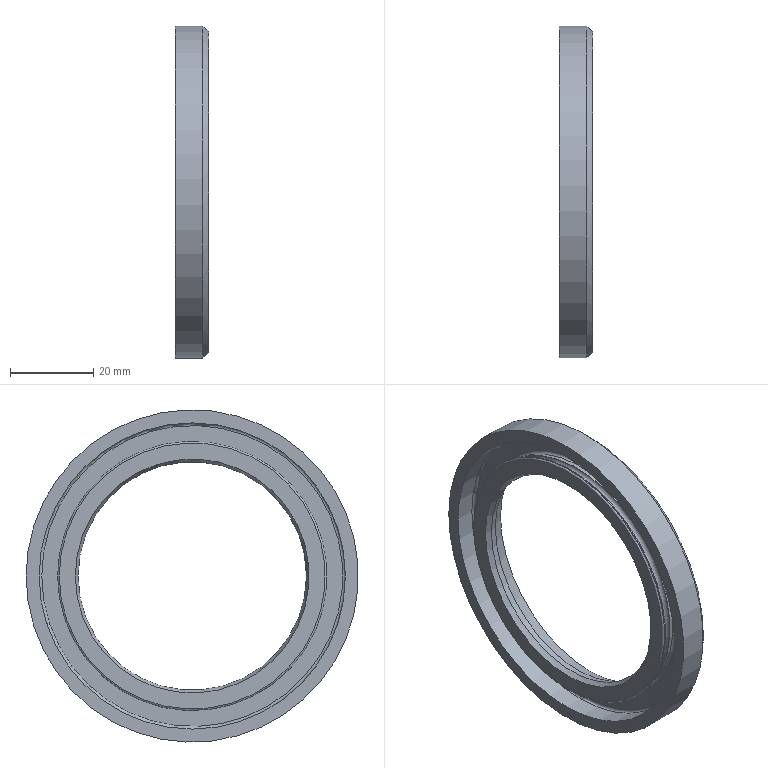Part | STEP file | Housing | 1 solid | 31 faces | box 8 x 80 x 80 mm | volume 10893 mm3 | plane 11 | cylinder 9 | torus 7 | cone 4 | commonest cylinder face diameters 67.5 x2 63.25 x1 64.85 x1 71.75 x1 73.75 x1 76.597 x1
STEP:
#1=CARTESIAN_POINT('',(8.,33.75,0.));
#2=VERTEX_POINT('',#1);
#3=CARTESIAN_POINT('',(8.,0.,0.));
#4=DIRECTION('',(1.,0.,0.));
#5=DIRECTION('',(0.,1.,0.));
#6=AXIS2_PLACEMENT_3D('',#3,#4,#5);
#7=CIRCLE('',#6,33.75);
#8=EDGE_CURVE('',#2,#2,#7,.T.);
#9=ORIENTED_EDGE('',*,*,#8,.T.);
#10=EDGE_LOOP('',(#9));
#11=FACE_BOUND('',#10,.T.);
#12=CARTESIAN_POINT('',(8.,30.393,0.));
#13=VERTEX_POINT('',#12);
#14=CARTESIAN_POINT('',(8.,0.,0.));
#15=DIRECTION('',(1.,0.,0.));
#16=DIRECTION('',(0.,1.,0.));
#17=AXIS2_PLACEMENT_3D('',#14,#15,#16);
#18=CIRCLE('',#17,30.393);
#19=EDGE_CURVE('',#13,#13,#18,.F.);
#20=ORIENTED_EDGE('',*,*,#19,.T.);
#21=EDGE_LOOP('',(#20));
#22=FACE_BOUND('',#21,.T.);
#23=CARTESIAN_POINT('',(8.,0.,0.));
#24=DIRECTION('',(1.,0.,0.));
#25=DIRECTION('',(0.,1.,0.));
#26=AXIS2_PLACEMENT_3D('',#23,#24,#25);
#27=PLANE('',#26);
#28=ADVANCED_FACE('',(#11,#22),#27,.T.);
#29=CARTESIAN_POINT('',(4.,28.15,0.));
#30=VERTEX_POINT('',#29);
#31=CARTESIAN_POINT('',(4.,0.,0.));
#32=DIRECTION('',(1.,0.,0.));
#33=DIRECTION('',(0.,1.,0.));
#34=AXIS2_PLACEMENT_3D('',#31,#32,#33);
#35=CIRCLE('',#34,28.15);
#36=EDGE_CURVE('',#30,#30,#35,.T.);
#37=ORIENTED_EDGE('',*,*,#36,.T.);
#38=EDGE_LOOP('',(#37));
#39=FACE_OUTER_BOUND('',#38,.T.);
#40=CARTESIAN_POINT('',(2.,27.5,0.));
#41=VERTEX_POINT('',#40);
#42=CARTESIAN_POINT('',(2.,0.,0.));
#43=DIRECTION('',(1.,0.,0.));
#44=DIRECTION('',(0.,1.,0.));
#45=AXIS2_PLACEMENT_3D('',#42,#43,#44);
#46=CIRCLE('',#45,27.5);
#47=EDGE_CURVE('',#41,#41,#46,.T.);
#48=ORIENTED_EDGE('',*,*,#47,.F.);
#49=EDGE_LOOP('',(#48));
#50=FACE_OUTER_BOUND('',#49,.T.);
#51=CARTESIAN_POINT('',(3.,0.,0.));
#52=DIRECTION('',(1.,0.,0.));
#53=DIRECTION('',(0.,1.,0.));
#54=AXIS2_PLACEMENT_3D('',#51,#52,#53);
#55=CONICAL_SURFACE('',#54,27.825,0.3142);
#56=ADVANCED_FACE('',(#39,#50),#55,.F.);
#57=CARTESIAN_POINT('',(4.,28.442,0.));
#58=VERTEX_POINT('',#57);
#59=CARTESIAN_POINT('',(4.,0.,0.));
#60=DIRECTION('',(1.,0.,0.));
#61=DIRECTION('',(0.,1.,0.));
#62=AXIS2_PLACEMENT_3D('',#59,#60,#61);
#63=CIRCLE('',#62,28.442);
#64=EDGE_CURVE('',#58,#58,#63,.T.);
#65=ORIENTED_EDGE('',*,*,#64,.T.);
#66=EDGE_LOOP('',(#65));
#67=FACE_BOUND('',#66,.T.);
#68=ORIENTED_EDGE('',*,*,#36,.F.);
#69=EDGE_LOOP('',(#68));
#70=FACE_BOUND('',#69,.T.);
#71=CARTESIAN_POINT('',(4.,0.,0.));
#72=DIRECTION('',(-1.,0.,0.));
#73=DIRECTION('',(0.,1.,0.));
#74=AXIS2_PLACEMENT_3D('',#71,#72,#73);
#75=PLANE('',#74);
#76=ADVANCED_FACE('',(#67,#70),#75,.F.);
#77=ORIENTED_EDGE('',*,*,#19,.F.);
#78=EDGE_LOOP('',(#77));
#79=FACE_OUTER_BOUND('',#78,.T.);
#80=ORIENTED_EDGE('',*,*,#64,.F.);
#81=EDGE_LOOP('',(#80));
#82=FACE_OUTER_BOUND('',#81,.T.);
#83=CARTESIAN_POINT('',(6.,0.,0.));
#84=DIRECTION('',(1.,0.,0.));
#85=DIRECTION('',(0.,1.,0.));
#86=AXIS2_PLACEMENT_3D('',#83,#84,#85);
#87=CONICAL_SURFACE('',#86,29.418,0.4538);
#88=ADVANCED_FACE('',(#79,#82),#87,.F.);
#89=ORIENTED_EDGE('',*,*,#8,.F.);
#90=EDGE_LOOP('',(#89));
#91=FACE_OUTER_BOUND('',#90,.T.);
#92=CARTESIAN_POINT('',(7.36,33.75,0.));
#93=VERTEX_POINT('',#92);
#94=CARTESIAN_POINT('',(7.36,0.,0.));
#95=DIRECTION('',(1.,0.,0.));
#96=DIRECTION('',(0.,1.,0.));
#97=AXIS2_PLACEMENT_3D('',#94,#95,#96);
#98=CIRCLE('',#97,33.75);
#99=EDGE_CURVE('',#93,#93,#98,.T.);
#100=ORIENTED_EDGE('',*,*,#99,.T.);
#101=EDGE_LOOP('',(#100));
#102=FACE_OUTER_BOUND('',#101,.T.);
#103=CARTESIAN_POINT('',(8.,0.,0.));
#104=DIRECTION('',(1.,0.,0.));
#105=DIRECTION('',(0.,1.,0.));
#106=AXIS2_PLACEMENT_3D('',#103,#104,#105);
#107=CYLINDRICAL_SURFACE('',#106,33.75);
#108=ADVANCED_FACE('',(#91,#102),#107,.T.);
#109=ORIENTED_EDGE('',*,*,#47,.T.);
#110=EDGE_LOOP('',(#109));
#111=FACE_OUTER_BOUND('',#110,.T.);
#112=CARTESIAN_POINT('',(0.64,28.163,0.));
#113=VERTEX_POINT('',#112);
#114=CARTESIAN_POINT('',(0.64,0.,0.));
#115=DIRECTION('',(1.,0.,0.));
#116=DIRECTION('',(0.,1.,0.));
#117=AXIS2_PLACEMENT_3D('',#114,#115,#116);
#118=CIRCLE('',#117,28.163);
#119=EDGE_CURVE('',#113,#113,#118,.T.);
#120=ORIENTED_EDGE('',*,*,#119,.F.);
#121=EDGE_LOOP('',(#120));
#122=FACE_OUTER_BOUND('',#121,.T.);
#123=CARTESIAN_POINT('',(1.32,0.,0.));
#124=DIRECTION('',(-1.,0.,0.));
#125=DIRECTION('',(0.,-1.,0.));
#126=AXIS2_PLACEMENT_3D('',#123,#124,#125);
#127=CONICAL_SURFACE('',#126,27.832,0.4538);
#128=ADVANCED_FACE('',(#111,#122),#127,.F.);
#129=CARTESIAN_POINT('',(7.36,35.875,0.));
#130=VERTEX_POINT('',#129);
#131=CARTESIAN_POINT('',(7.36,0.,0.));
#132=DIRECTION('',(1.,0.,0.));
#133=DIRECTION('',(0.,1.,0.));
#134=AXIS2_PLACEMENT_3D('',#131,#132,#133);
#135=CIRCLE('',#134,35.875);
#136=EDGE_CURVE('',#130,#130,#135,.T.);
#137=ORIENTED_EDGE('',*,*,#136,.T.);
#138=EDGE_LOOP('',(#137));
#139=FACE_BOUND('',#138,.T.);
#140=ORIENTED_EDGE('',*,*,#99,.F.);
#141=EDGE_LOOP('',(#140));
#142=FACE_BOUND('',#141,.T.);
#143=CARTESIAN_POINT('',(7.36,0.,0.));
#144=DIRECTION('',(-1.,0.,0.));
#145=DIRECTION('',(0.,1.,0.));
#146=AXIS2_PLACEMENT_3D('',#143,#144,#145);
#147=PLANE('',#146);
#148=ADVANCED_FACE('',(#139,#142),#147,.F.);
#149=CARTESIAN_POINT('',(0.64,32.025,0.));
#150=VERTEX_POINT('',#149);
#151=CARTESIAN_POINT('',(0.64,0.,0.));
#152=DIRECTION('',(1.,0.,0.));
#153=DIRECTION('',(0.,1.,0.));
#154=AXIS2_PLACEMENT_3D('',#151,#152,#153);
#155=CIRCLE('',#154,32.025);
#156=EDGE_CURVE('',#150,#150,#155,.T.);
#157=ORIENTED_EDGE('',*,*,#156,.F.);
#158=EDGE_LOOP('',(#157));
#159=FACE_BOUND('',#158,.T.);
#160=ORIENTED_EDGE('',*,*,#119,.T.);
#161=EDGE_LOOP('',(#160));
#162=FACE_BOUND('',#161,.T.);
#163=CARTESIAN_POINT('',(0.64,0.,0.));
#164=DIRECTION('',(1.,0.,0.));
#165=DIRECTION('',(0.,1.,0.));
#166=AXIS2_PLACEMENT_3D('',#163,#164,#165);
#167=PLANE('',#166);
#168=ADVANCED_FACE('',(#159,#162),#167,.F.);
#169=CARTESIAN_POINT('',(8.,35.875,0.));
#170=VERTEX_POINT('',#169);
#171=CARTESIAN_POINT('',(8.,0.,0.));
#172=DIRECTION('',(1.,0.,0.));
#173=DIRECTION('',(0.,1.,0.));
#174=AXIS2_PLACEMENT_3D('',#171,#172,#173);
#175=CIRCLE('',#174,35.875);
#176=EDGE_CURVE('',#170,#170,#175,.F.);
#177=ORIENTED_EDGE('',*,*,#176,.F.);
#178=EDGE_LOOP('',(#177));
#179=FACE_OUTER_BOUND('',#178,.T.);
#180=ORIENTED_EDGE('',*,*,#136,.F.);
#181=EDGE_LOOP('',(#180));
#182=FACE_OUTER_BOUND('',#181,.T.);
#183=CARTESIAN_POINT('',(7.36,0.,0.));
#184=DIRECTION('',(1.,0.,0.));
#185=DIRECTION('',(0.,1.,0.));
#186=AXIS2_PLACEMENT_3D('',#183,#184,#185);
#187=CYLINDRICAL_SURFACE('',#186,35.875);
#188=ADVANCED_FACE('',(#179,#182),#187,.F.);
#189=CARTESIAN_POINT('',(1.04,32.425,0.));
#190=VERTEX_POINT('',#189);
#191=CARTESIAN_POINT('',(1.04,0.,0.));
#192=DIRECTION('',(1.,0.,0.));
#193=DIRECTION('',(0.,1.,0.));
#194=AXIS2_PLACEMENT_3D('',#191,#192,#193);
#195=CIRCLE('',#194,32.425);
#196=EDGE_CURVE('',#190,#190,#195,.T.);
#197=ORIENTED_EDGE('',*,*,#196,.F.);
#198=EDGE_LOOP('',(#197));
#199=FACE_OUTER_BOUND('',#198,.T.);
#200=ORIENTED_EDGE('',*,*,#156,.T.);
#201=EDGE_LOOP('',(#200));
#202=FACE_OUTER_BOUND('',#201,.T.);
#203=CARTESIAN_POINT('',(1.04,0.,0.));
#204=DIRECTION('',(1.,0.,0.));
#205=DIRECTION('',(0.,1.,0.));
#206=AXIS2_PLACEMENT_3D('',#203,#204,#205);
#207=TOROIDAL_SURFACE('',#206,32.025,0.4);
#208=ADVANCED_FACE('',(#199,#202),#207,.T.);
#209=CARTESIAN_POINT('',(8.,38.64,0.));
#210=VERTEX_POINT('',#209);
#211=CARTESIAN_POINT('',(8.,0.,0.));
#212=DIRECTION('',(1.,0.,0.));
#213=DIRECTION('',(0.,1.,0.));
#214=AXIS2_PLACEMENT_3D('',#211,#212,#213);
#215=CIRCLE('',#214,38.64);
#216=EDGE_CURVE('',#210,#210,#215,.T.);
#217=ORIENTED_EDGE('',*,*,#216,.T.);
#218=EDGE_LOOP('',(#217));
#219=FACE_BOUND('',#218,.T.);
#220=ORIENTED_EDGE('',*,*,#176,.T.);
#221=EDGE_LOOP('',(#220));
#222=FACE_BOUND('',#221,.T.);
#223=CARTESIAN_POINT('',(8.,0.,0.));
#224=DIRECTION('',(1.,0.,0.));
#225=DIRECTION('',(0.,1.,0.));
#226=AXIS2_PLACEMENT_3D('',#223,#224,#225);
#227=PLANE('',#226);
#228=ADVANCED_FACE('',(#219,#222),#227,.T.);
#229=CARTESIAN_POINT('',(1.2,32.425,0.));
#230=VERTEX_POINT('',#229);
#231=CARTESIAN_POINT('',(1.2,0.,0.));
#232=DIRECTION('',(1.,0.,0.));
#233=DIRECTION('',(0.,1.,0.));
#234=AXIS2_PLACEMENT_3D('',#231,#232,#233);
#235=CIRCLE('',#234,32.425);
#236=EDGE_CURVE('',#230,#230,#235,.T.);
#237=ORIENTED_EDGE('',*,*,#236,.F.);
#238=EDGE_LOOP('',(#237));
#239=FACE_OUTER_BOUND('',#238,.T.);
#240=ORIENTED_EDGE('',*,*,#196,.T.);
#241=EDGE_LOOP('',(#240));
#242=FACE_OUTER_BOUND('',#241,.T.);
#243=CARTESIAN_POINT('',(0.64,0.,0.));
#244=DIRECTION('',(1.,0.,0.));
#245=DIRECTION('',(0.,1.,0.));
#246=AXIS2_PLACEMENT_3D('',#243,#244,#245);
#247=CYLINDRICAL_SURFACE('',#246,32.425);
#248=ADVANCED_FACE('',(#239,#242),#247,.T.);
#249=CARTESIAN_POINT('',(6.64,40.,0.));
#250=VERTEX_POINT('',#249);
#251=CARTESIAN_POINT('',(6.64,0.,0.));
#252=DIRECTION('',(1.,0.,0.));
#253=DIRECTION('',(0.,1.,0.));
#254=AXIS2_PLACEMENT_3D('',#251,#252,#253);
#255=CIRCLE('',#254,40.);
#256=EDGE_CURVE('',#250,#250,#255,.T.);
#257=ORIENTED_EDGE('',*,*,#256,.F.);
#258=EDGE_LOOP('',(#257));
#259=FACE_OUTER_BOUND('',#258,.T.);
#260=CARTESIAN_POINT('',(0.,40.,0.));
#261=VERTEX_POINT('',#260);
#262=CARTESIAN_POINT('',(0.,0.,0.));
#263=DIRECTION('',(1.,0.,0.));
#264=DIRECTION('',(0.,1.,0.));
#265=AXIS2_PLACEMENT_3D('',#262,#263,#264);
#266=CIRCLE('',#265,40.);
#267=EDGE_CURVE('',#261,#261,#266,.T.);
#268=ORIENTED_EDGE('',*,*,#267,.T.);
#269=EDGE_LOOP('',(#268));
#270=FACE_OUTER_BOUND('',#269,.T.);
#271=CARTESIAN_POINT('',(0.,0.,0.));
#272=DIRECTION('',(1.,0.,0.));
#273=DIRECTION('',(0.,1.,0.));
#274=AXIS2_PLACEMENT_3D('',#271,#272,#273);
#275=CYLINDRICAL_SURFACE('',#274,40.);
#276=ADVANCED_FACE('',(#259,#270),#275,.T.);
#277=CARTESIAN_POINT('',(1.6,32.025,0.));
#278=VERTEX_POINT('',#277);
#279=CARTESIAN_POINT('',(1.6,0.,0.));
#280=DIRECTION('',(1.,0.,0.));
#281=DIRECTION('',(0.,1.,0.));
#282=AXIS2_PLACEMENT_3D('',#279,#280,#281);
#283=CIRCLE('',#282,32.025);
#284=EDGE_CURVE('',#278,#278,#283,.T.);
#285=ORIENTED_EDGE('',*,*,#284,.F.);
#286=EDGE_LOOP('',(#285));
#287=FACE_OUTER_BOUND('',#286,.T.);
#288=ORIENTED_EDGE('',*,*,#236,.T.);
#289=EDGE_LOOP('',(#288));
#290=FACE_OUTER_BOUND('',#289,.T.);
#291=CARTESIAN_POINT('',(1.2,0.,0.));
#292=DIRECTION('',(1.,0.,0.));
#293=DIRECTION('',(0.,1.,0.));
#294=AXIS2_PLACEMENT_3D('',#291,#292,#293);
#295=TOROIDAL_SURFACE('',#294,32.025,0.4);
#296=ADVANCED_FACE('',(#287,#290),#295,.T.);
#297=ORIENTED_EDGE('',*,*,#267,.F.);
#298=EDGE_LOOP('',(#297));
#299=FACE_BOUND('',#298,.T.);
#300=CARTESIAN_POINT('',(0.,36.875,0.));
#301=VERTEX_POINT('',#300);
#302=CARTESIAN_POINT('',(0.,0.,0.));
#303=DIRECTION('',(1.,0.,0.));
#304=DIRECTION('',(0.,1.,0.));
#305=AXIS2_PLACEMENT_3D('',#302,#303,#304);
#306=CIRCLE('',#305,36.875);
#307=EDGE_CURVE('',#301,#301,#306,.T.);
#308=ORIENTED_EDGE('',*,*,#307,.T.);
#309=EDGE_LOOP('',(#308));
#310=FACE_BOUND('',#309,.T.);
#311=CARTESIAN_POINT('',(0.,0.,0.));
#312=DIRECTION('',(-1.,0.,0.));
#313=DIRECTION('',(0.,1.,0.));
#314=AXIS2_PLACEMENT_3D('',#311,#312,#313);
#315=PLANE('',#314);
#316=ADVANCED_FACE('',(#299,#310),#315,.T.);
#317=ORIENTED_EDGE('',*,*,#284,.T.);
#318=EDGE_LOOP('',(#317));
#319=FACE_BOUND('',#318,.T.);
#320=CARTESIAN_POINT('',(1.6,31.625,0.));
#321=VERTEX_POINT('',#320);
#322=CARTESIAN_POINT('',(1.6,0.,0.));
#323=DIRECTION('',(1.,0.,0.));
#324=DIRECTION('',(0.,1.,0.));
#325=AXIS2_PLACEMENT_3D('',#322,#323,#324);
#326=CIRCLE('',#325,31.625);
#327=EDGE_CURVE('',#321,#321,#326,.F.);
#328=ORIENTED_EDGE('',*,*,#327,.T.);
#329=EDGE_LOOP('',(#328));
#330=FACE_BOUND('',#329,.T.);
#331=CARTESIAN_POINT('',(1.6,0.,0.));
#332=DIRECTION('',(1.,0.,0.));
#333=DIRECTION('',(0.,1.,0.));
#334=AXIS2_PLACEMENT_3D('',#331,#332,#333);
#335=PLANE('',#334);
#336=ADVANCED_FACE('',(#319,#330),#335,.T.);
#337=CARTESIAN_POINT('',(4.72,36.875,0.));
#338=VERTEX_POINT('',#337);
#339=CARTESIAN_POINT('',(4.72,0.,0.));
#340=DIRECTION('',(1.,0.,0.));
#341=DIRECTION('',(0.,1.,0.));
#342=AXIS2_PLACEMENT_3D('',#339,#340,#341);
#343=CIRCLE('',#342,36.875);
#344=EDGE_CURVE('',#338,#338,#343,.T.);
#345=ORIENTED_EDGE('',*,*,#344,.T.);
#346=EDGE_LOOP('',(#345));
#347=FACE_OUTER_BOUND('',#346,.T.);
#348=ORIENTED_EDGE('',*,*,#307,.F.);
#349=EDGE_LOOP('',(#348));
#350=FACE_OUTER_BOUND('',#349,.T.);
#351=CARTESIAN_POINT('',(0.,0.,0.));
#352=DIRECTION('',(1.,0.,0.));
#353=DIRECTION('',(0.,1.,0.));
#354=AXIS2_PLACEMENT_3D('',#351,#352,#353);
#355=CYLINDRICAL_SURFACE('',#354,36.875);
#356=ADVANCED_FACE('',(#347,#350),#355,.F.);
#357=CARTESIAN_POINT('',(3.68,31.625,0.));
#358=VERTEX_POINT('',#357);
#359=CARTESIAN_POINT('',(3.68,0.,0.));
#360=DIRECTION('',(1.,0.,0.));
#361=DIRECTION('',(0.,1.,0.));
#362=AXIS2_PLACEMENT_3D('',#359,#360,#361);
#363=CIRCLE('',#362,31.625);
#364=EDGE_CURVE('',#358,#358,#363,.T.);
#365=ORIENTED_EDGE('',*,*,#364,.F.);
#366=EDGE_LOOP('',(#365));
#367=FACE_OUTER_BOUND('',#366,.T.);
#368=ORIENTED_EDGE('',*,*,#327,.F.);
#369=EDGE_LOOP('',(#368));
#370=FACE_OUTER_BOUND('',#369,.T.);
#371=CARTESIAN_POINT('',(2.64,0.,0.));
#372=DIRECTION('',(1.,0.,0.));
#373=DIRECTION('',(0.,1.,0.));
#374=AXIS2_PLACEMENT_3D('',#371,#372,#373);
#375=TOROIDAL_SURFACE('',#374,31.625,1.04);
#376=ADVANCED_FACE('',(#367,#370),#375,.F.);
#377=CARTESIAN_POINT('',(5.36,36.235,0.));
#378=VERTEX_POINT('',#377);
#379=CARTESIAN_POINT('',(5.36,0.,0.));
#380=DIRECTION('',(1.,0.,0.));
#381=DIRECTION('',(0.,1.,0.));
#382=AXIS2_PLACEMENT_3D('',#379,#380,#381);
#383=CIRCLE('',#382,36.235);
#384=EDGE_CURVE('',#378,#378,#383,.T.);
#385=ORIENTED_EDGE('',*,*,#384,.F.);
#386=EDGE_LOOP('',(#385));
#387=FACE_BOUND('',#386,.T.);
#388=CARTESIAN_POINT('',(5.36,32.265,0.));
#389=VERTEX_POINT('',#388);
#390=CARTESIAN_POINT('',(5.36,0.,0.));
#391=DIRECTION('',(1.,0.,0.));
#392=DIRECTION('',(0.,1.,0.));
#393=AXIS2_PLACEMENT_3D('',#390,#391,#392);
#394=CIRCLE('',#393,32.265);
#395=EDGE_CURVE('',#389,#389,#394,.T.);
#396=ORIENTED_EDGE('',*,*,#395,.T.);
#397=EDGE_LOOP('',(#396));
#398=FACE_BOUND('',#397,.T.);
#399=CARTESIAN_POINT('',(5.36,0.,0.));
#400=DIRECTION('',(1.,0.,0.));
#401=DIRECTION('',(0.,1.,0.));
#402=AXIS2_PLACEMENT_3D('',#399,#400,#401);
#403=PLANE('',#402);
#404=ADVANCED_FACE('',(#387,#398),#403,.F.);
#405=CARTESIAN_POINT('',(4.72,31.625,0.));
#406=VERTEX_POINT('',#405);
#407=CARTESIAN_POINT('',(4.72,0.,0.));
#408=DIRECTION('',(1.,0.,0.));
#409=DIRECTION('',(0.,1.,0.));
#410=AXIS2_PLACEMENT_3D('',#407,#408,#409);
#411=CIRCLE('',#410,31.625);
#412=EDGE_CURVE('',#406,#406,#411,.T.);
#413=ORIENTED_EDGE('',*,*,#412,.F.);
#414=EDGE_LOOP('',(#413));
#415=FACE_OUTER_BOUND('',#414,.T.);
#416=ORIENTED_EDGE('',*,*,#364,.T.);
#417=EDGE_LOOP('',(#416));
#418=FACE_OUTER_BOUND('',#417,.T.);
#419=CARTESIAN_POINT('',(5.36,0.,0.));
#420=DIRECTION('',(1.,0.,0.));
#421=DIRECTION('',(0.,1.,0.));
#422=AXIS2_PLACEMENT_3D('',#419,#420,#421);
#423=CYLINDRICAL_SURFACE('',#422,31.625);
#424=ADVANCED_FACE('',(#415,#418),#423,.T.);
#425=ORIENTED_EDGE('',*,*,#384,.T.);
#426=EDGE_LOOP('',(#425));
#427=FACE_OUTER_BOUND('',#426,.T.);
#428=ORIENTED_EDGE('',*,*,#344,.F.);
#429=EDGE_LOOP('',(#428));
#430=FACE_OUTER_BOUND('',#429,.T.);
#431=CARTESIAN_POINT('',(4.72,0.,0.));
#432=DIRECTION('',(1.,0.,0.));
#433=DIRECTION('',(0.,1.,0.));
#434=AXIS2_PLACEMENT_3D('',#431,#432,#433);
#435=TOROIDAL_SURFACE('',#434,36.235,0.64);
#436=ADVANCED_FACE('',(#427,#430),#435,.F.);
#437=ORIENTED_EDGE('',*,*,#395,.F.);
#438=EDGE_LOOP('',(#437));
#439=FACE_OUTER_BOUND('',#438,.T.);
#440=ORIENTED_EDGE('',*,*,#412,.T.);
#441=EDGE_LOOP('',(#440));
#442=FACE_OUTER_BOUND('',#441,.T.);
#443=CARTESIAN_POINT('',(4.72,0.,0.));
#444=DIRECTION('',(1.,0.,0.));
#445=DIRECTION('',(0.,1.,0.));
#446=AXIS2_PLACEMENT_3D('',#443,#444,#445);
#447=TOROIDAL_SURFACE('',#446,32.265,0.64);
#448=ADVANCED_FACE('',(#439,#442),#447,.F.);
#449=ORIENTED_EDGE('',*,*,#216,.F.);
#450=EDGE_LOOP('',(#449));
#451=FACE_OUTER_BOUND('',#450,.T.);
#452=ORIENTED_EDGE('',*,*,#256,.T.);
#453=EDGE_LOOP('',(#452));
#454=FACE_OUTER_BOUND('',#453,.T.);
#455=CARTESIAN_POINT('',(7.32,0.,0.));
#456=DIRECTION('',(-1.,0.,0.));
#457=DIRECTION('',(0.,-1.,0.));
#458=AXIS2_PLACEMENT_3D('',#455,#456,#457);
#459=CONICAL_SURFACE('',#458,39.32,0.7854);
#460=ADVANCED_FACE('',(#451,#454),#459,.T.);
#461=CLOSED_SHELL('',(#28,#56,#76,#88,#108,#128,#148,#168,#188,#208,#228,#248,#276,#296,#316,#336,#356,#376,#404,#424,#436,#448,#460));
#462=CARTESIAN_POINT('',(1.36,38.962,0.));
#463=VERTEX_POINT('',#462);
#464=CARTESIAN_POINT('',(1.36,0.,0.));
#465=DIRECTION('',(1.,0.,0.));
#466=DIRECTION('',(0.,1.,0.));
#467=AXIS2_PLACEMENT_3D('',#464,#465,#466);
#468=CIRCLE('',#467,38.962);
#469=EDGE_CURVE('',#463,#463,#468,.T.);
#470=ORIENTED_EDGE('',*,*,#469,.T.);
#471=EDGE_LOOP('',(#470));
#472=FACE_BOUND('',#471,.T.);
#473=CARTESIAN_POINT('',(1.36,38.298,0.));
#474=VERTEX_POINT('',#473);
#475=CARTESIAN_POINT('',(1.36,0.,0.));
#476=DIRECTION('',(1.,0.,0.));
#477=DIRECTION('',(0.,1.,0.));
#478=AXIS2_PLACEMENT_3D('',#475,#476,#477);
#479=CIRCLE('',#478,38.298);
#480=EDGE_CURVE('',#474,#474,#479,.T.);
#481=ORIENTED_EDGE('',*,*,#480,.F.);
#482=EDGE_LOOP('',(#481));
#483=FACE_BOUND('',#482,.T.);
#484=CARTESIAN_POINT('',(1.36,0.,0.));
#485=DIRECTION('',(-1.,0.,0.));
#486=DIRECTION('',(0.,1.,0.));
#487=AXIS2_PLACEMENT_3D('',#484,#485,#486);
#488=PLANE('',#487);
#489=ADVANCED_FACE('',(#472,#483),#488,.F.);
#490=CARTESIAN_POINT('',(5.976,38.962,0.));
#491=VERTEX_POINT('',#490);
#492=CARTESIAN_POINT('',(5.976,0.,0.));
#493=DIRECTION('',(1.,0.,0.));
#494=DIRECTION('',(0.,1.,0.));
#495=AXIS2_PLACEMENT_3D('',#492,#493,#494);
#496=CIRCLE('',#495,38.962);
#497=EDGE_CURVE('',#491,#491,#496,.T.);
#498=ORIENTED_EDGE('',*,*,#497,.T.);
#499=EDGE_LOOP('',(#498));
#500=FACE_OUTER_BOUND('',#499,.T.);
#501=ORIENTED_EDGE('',*,*,#469,.F.);
#502=EDGE_LOOP('',(#501));
#503=FACE_OUTER_BOUND('',#502,.T.);
#504=CARTESIAN_POINT('',(1.36,0.,0.));
#505=DIRECTION('',(1.,0.,0.));
#506=DIRECTION('',(0.,1.,0.));
#507=AXIS2_PLACEMENT_3D('',#504,#505,#506);
#508=CYLINDRICAL_SURFACE('',#507,38.962);
#509=ADVANCED_FACE('',(#500,#503),#508,.F.);
#510=CARTESIAN_POINT('',(5.644,38.298,0.));
#511=VERTEX_POINT('',#510);
#512=CARTESIAN_POINT('',(5.644,0.,0.));
#513=DIRECTION('',(1.,0.,0.));
#514=DIRECTION('',(0.,1.,0.));
#515=AXIS2_PLACEMENT_3D('',#512,#513,#514);
#516=CIRCLE('',#515,38.298);
#517=EDGE_CURVE('',#511,#511,#516,.T.);
#518=ORIENTED_EDGE('',*,*,#517,.F.);
#519=EDGE_LOOP('',(#518));
#520=FACE_OUTER_BOUND('',#519,.T.);
#521=ORIENTED_EDGE('',*,*,#480,.T.);
#522=EDGE_LOOP('',(#521));
#523=FACE_OUTER_BOUND('',#522,.T.);
#524=CARTESIAN_POINT('',(5.644,0.,0.));
#525=DIRECTION('',(1.,0.,0.));
#526=DIRECTION('',(0.,1.,0.));
#527=AXIS2_PLACEMENT_3D('',#524,#525,#526);
#528=CYLINDRICAL_SURFACE('',#527,38.298);
#529=ADVANCED_FACE('',(#520,#523),#528,.T.);
#530=CARTESIAN_POINT('',(6.64,38.298,0.));
#531=VERTEX_POINT('',#530);
#532=CARTESIAN_POINT('',(6.64,0.,0.));
#533=DIRECTION('',(1.,0.,0.));
#534=DIRECTION('',(0.,1.,0.));
#535=AXIS2_PLACEMENT_3D('',#532,#533,#534);
#536=CIRCLE('',#535,38.298);
#537=EDGE_CURVE('',#531,#531,#536,.T.);
#538=ORIENTED_EDGE('',*,*,#537,.T.);
#539=EDGE_LOOP('',(#538));
#540=FACE_OUTER_BOUND('',#539,.T.);
#541=ORIENTED_EDGE('',*,*,#497,.F.);
#542=EDGE_LOOP('',(#541));
#543=FACE_OUTER_BOUND('',#542,.T.);
#544=CARTESIAN_POINT('',(5.976,0.,0.));
#545=DIRECTION('',(1.,0.,0.));
#546=DIRECTION('',(0.,1.,0.));
#547=AXIS2_PLACEMENT_3D('',#544,#545,#546);
#548=TOROIDAL_SURFACE('',#547,38.298,0.664);
#549=ADVANCED_FACE('',(#540,#543),#548,.F.);
#550=CARTESIAN_POINT('',(5.976,37.966,0.));
#551=VERTEX_POINT('',#550);
#552=CARTESIAN_POINT('',(5.976,0.,0.));
#553=DIRECTION('',(1.,0.,0.));
#554=DIRECTION('',(0.,1.,0.));
#555=AXIS2_PLACEMENT_3D('',#552,#553,#554);
#556=CIRCLE('',#555,37.966);
#557=EDGE_CURVE('',#551,#551,#556,.T.);
#558=ORIENTED_EDGE('',*,*,#557,.F.);
#559=EDGE_LOOP('',(#558));
#560=FACE_OUTER_BOUND('',#559,.T.);
#561=ORIENTED_EDGE('',*,*,#517,.T.);
#562=EDGE_LOOP('',(#561));
#563=FACE_OUTER_BOUND('',#562,.T.);
#564=CARTESIAN_POINT('',(5.644,0.,0.));
#565=DIRECTION('',(1.,0.,0.));
#566=DIRECTION('',(0.,1.,0.));
#567=AXIS2_PLACEMENT_3D('',#564,#565,#566);
#568=TOROIDAL_SURFACE('',#567,37.967,0.332);
#569=ADVANCED_FACE('',(#560,#563),#568,.T.);
#570=ORIENTED_EDGE('',*,*,#537,.F.);
#571=EDGE_LOOP('',(#570));
#572=FACE_BOUND('',#571,.T.);
#573=CARTESIAN_POINT('',(6.64,33.75,0.));
#574=VERTEX_POINT('',#573);
#575=CARTESIAN_POINT('',(6.64,0.,0.));
#576=DIRECTION('',(1.,0.,0.));
#577=DIRECTION('',(0.,1.,0.));
#578=AXIS2_PLACEMENT_3D('',#575,#576,#577);
#579=CIRCLE('',#578,33.75);
#580=EDGE_CURVE('',#574,#574,#579,.T.);
#581=ORIENTED_EDGE('',*,*,#580,.T.);
#582=EDGE_LOOP('',(#581));
#583=FACE_BOUND('',#582,.T.);
#584=CARTESIAN_POINT('',(6.64,0.,0.));
#585=DIRECTION('',(1.,0.,0.));
#586=DIRECTION('',(0.,1.,0.));
#587=AXIS2_PLACEMENT_3D('',#584,#585,#586);
#588=PLANE('',#587);
#589=ADVANCED_FACE('',(#572,#583),#588,.F.);
#590=ORIENTED_EDGE('',*,*,#557,.T.);
#591=EDGE_LOOP('',(#590));
#592=FACE_BOUND('',#591,.T.);
#593=CARTESIAN_POINT('',(5.976,33.75,0.));
#594=VERTEX_POINT('',#593);
#595=CARTESIAN_POINT('',(5.976,0.,0.));
#596=DIRECTION('',(1.,0.,0.));
#597=DIRECTION('',(0.,1.,0.));
#598=AXIS2_PLACEMENT_3D('',#595,#596,#597);
#599=CIRCLE('',#598,33.75);
#600=EDGE_CURVE('',#594,#594,#599,.T.);
#601=ORIENTED_EDGE('',*,*,#600,.F.);
#602=EDGE_LOOP('',(#601));
#603=FACE_BOUND('',#602,.T.);
#604=CARTESIAN_POINT('',(5.976,0.,0.));
#605=DIRECTION('',(-1.,0.,0.));
#606=DIRECTION('',(0.,1.,0.));
#607=AXIS2_PLACEMENT_3D('',#604,#605,#606);
#608=PLANE('',#607);
#609=ADVANCED_FACE('',(#592,#603),#608,.F.);
#610=ORIENTED_EDGE('',*,*,#580,.F.);
#611=EDGE_LOOP('',(#610));
#612=FACE_OUTER_BOUND('',#611,.T.);
#613=ORIENTED_EDGE('',*,*,#600,.T.);
#614=EDGE_LOOP('',(#613));
#615=FACE_OUTER_BOUND('',#614,.T.);
#616=CARTESIAN_POINT('',(6.64,0.,0.));
#617=DIRECTION('',(1.,0.,0.));
#618=DIRECTION('',(0.,1.,0.));
#619=AXIS2_PLACEMENT_3D('',#616,#617,#618);
#620=CYLINDRICAL_SURFACE('',#619,33.75);
#621=ADVANCED_FACE('',(#612,#615),#620,.T.);
#622=CLOSED_SHELL('',(#489,#509,#529,#549,#569,#589,#609,#621));
#623=ORIENTED_CLOSED_SHELL('',*,#622,.T.);
#624=BREP_WITH_VOIDS('',#461,(#623));
#625=(LENGTH_UNIT()NAMED_UNIT(*)SI_UNIT(.MILLI.,.METRE.));
#626=UNCERTAINTY_MEASURE_WITH_UNIT(LENGTH_MEASURE(0.00001),#625,'','');
#627=(NAMED_UNIT(*)PLANE_ANGLE_UNIT()SI_UNIT($,.RADIAN.));
#628=(NAMED_UNIT(*)SI_UNIT($,.STERADIAN.)SOLID_ANGLE_UNIT());
#629=(GEOMETRIC_REPRESENTATION_CONTEXT(3)GLOBAL_UNCERTAINTY_ASSIGNED_CONTEXT((#626))GLOBAL_UNIT_ASSIGNED_CONTEXT((#625,#627,#628))REPRESENTATION_CONTEXT('',''));
#630=ADVANCED_BREP_SHAPE_REPRESENTATION('',(#624),#629);